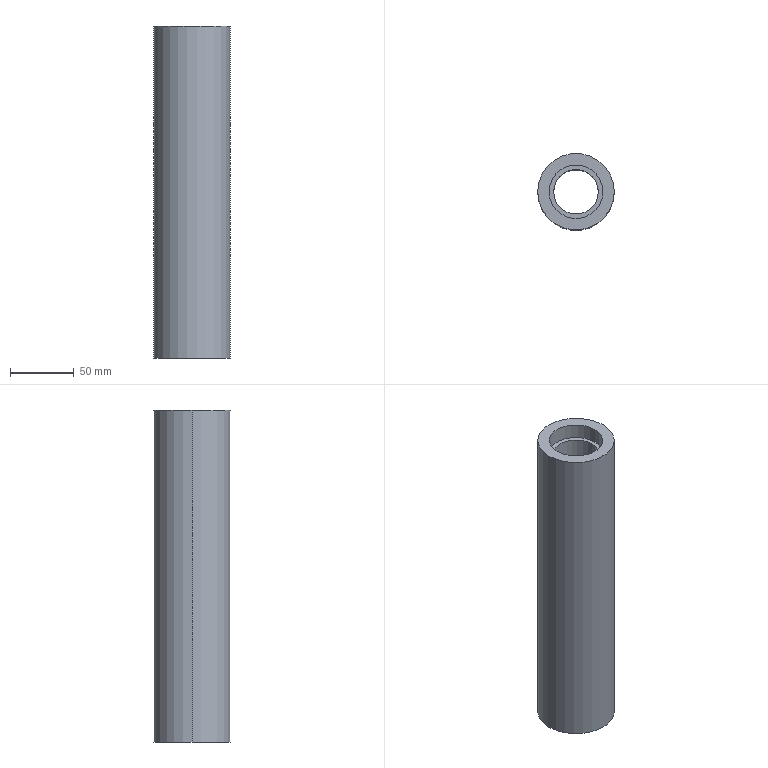Part | SolidWorks | features BaseBody 1 | 1 solid | 12 faces | box 60 x 60 x 260 mm | volume 474823 mm3 | cylinder 8 | plane 4 | commonest cylinder face diameters 42 x4 35 x2 60 x2
STEP:
#1=CARTESIAN_POINT('',(30.,0.,-130.));
#2=VERTEX_POINT('',#1);
#3=CARTESIAN_POINT('',(-30.,0.,-130.));
#4=VERTEX_POINT('',#3);
#5=CARTESIAN_POINT('',(0.,0.,-130.));
#6=DIRECTION('',(0.,0.,1.));
#7=DIRECTION('',(1.,0.,0.));
#8=AXIS2_PLACEMENT_3D('',#5,#6,#7);
#9=CIRCLE('',#8,30.);
#10=EDGE_CURVE('',#2,#4,#9,.T.);
#11=ORIENTED_EDGE('',*,*,#10,.T.);
#12=CARTESIAN_POINT('',(-30.,0.,130.));
#13=VERTEX_POINT('',#12);
#14=CARTESIAN_POINT('',(-30.,0.,-130.));
#15=DIRECTION('',(0.,0.,1.));
#16=VECTOR('',#15,1000.);
#17=LINE('',#14,#16);
#18=EDGE_CURVE('',#4,#13,#17,.T.);
#19=ORIENTED_EDGE('',*,*,#18,.T.);
#20=CARTESIAN_POINT('',(30.,0.,130.));
#21=VERTEX_POINT('',#20);
#22=CARTESIAN_POINT('',(0.,0.,130.));
#23=DIRECTION('',(0.,0.,-1.));
#24=DIRECTION('',(1.,0.,0.));
#25=AXIS2_PLACEMENT_3D('',#22,#23,#24);
#26=CIRCLE('',#25,30.);
#27=EDGE_CURVE('',#13,#21,#26,.T.);
#28=ORIENTED_EDGE('',*,*,#27,.T.);
#29=CARTESIAN_POINT('',(30.,0.,-130.));
#30=DIRECTION('',(0.,0.,1.));
#31=VECTOR('',#30,1000.);
#32=LINE('',#29,#31);
#33=EDGE_CURVE('',#2,#21,#32,.T.);
#34=ORIENTED_EDGE('',*,*,#33,.F.);
#35=EDGE_LOOP('',(#11,#19,#28,#34));
#36=FACE_OUTER_BOUND('',#35,.T.);
#37=CARTESIAN_POINT('',(0.,0.,-130.));
#38=DIRECTION('',(0.,0.,1.));
#39=DIRECTION('',(1.,0.,0.));
#40=AXIS2_PLACEMENT_3D('',#37,#38,#39);
#41=CYLINDRICAL_SURFACE('',#40,30.);
#42=ADVANCED_FACE('',(#36),#41,.T.);
#43=CARTESIAN_POINT('',(21.,0.,-130.));
#44=VERTEX_POINT('',#43);
#45=CARTESIAN_POINT('',(-21.,0.,-130.));
#46=VERTEX_POINT('',#45);
#47=CARTESIAN_POINT('',(0.,0.,-130.));
#48=DIRECTION('',(0.,0.,-1.));
#49=DIRECTION('',(1.,0.,0.));
#50=AXIS2_PLACEMENT_3D('',#47,#48,#49);
#51=CIRCLE('',#50,21.);
#52=EDGE_CURVE('',#44,#46,#51,.T.);
#53=ORIENTED_EDGE('',*,*,#52,.T.);
#54=CARTESIAN_POINT('',(-21.,0.,-118.));
#55=VERTEX_POINT('',#54);
#56=CARTESIAN_POINT('',(-21.,0.,-130.));
#57=DIRECTION('',(0.,0.,1.));
#58=VECTOR('',#57,1000.);
#59=LINE('',#56,#58);
#60=EDGE_CURVE('',#46,#55,#59,.T.);
#61=ORIENTED_EDGE('',*,*,#60,.T.);
#62=CARTESIAN_POINT('',(21.,0.,-118.));
#63=VERTEX_POINT('',#62);
#64=CARTESIAN_POINT('',(0.,0.,-118.));
#65=DIRECTION('',(0.,0.,-1.));
#66=DIRECTION('',(1.,0.,0.));
#67=AXIS2_PLACEMENT_3D('',#64,#65,#66);
#68=CIRCLE('',#67,21.);
#69=EDGE_CURVE('',#63,#55,#68,.T.);
#70=ORIENTED_EDGE('',*,*,#69,.F.);
#71=CARTESIAN_POINT('',(21.,0.,-130.));
#72=DIRECTION('',(0.,0.,1.));
#73=VECTOR('',#72,1000.);
#74=LINE('',#71,#73);
#75=EDGE_CURVE('',#44,#63,#74,.T.);
#76=ORIENTED_EDGE('',*,*,#75,.F.);
#77=EDGE_LOOP('',(#53,#61,#70,#76));
#78=FACE_OUTER_BOUND('',#77,.T.);
#79=CARTESIAN_POINT('',(0.,0.,-130.));
#80=DIRECTION('',(0.,0.,1.));
#81=DIRECTION('',(1.,0.,0.));
#82=AXIS2_PLACEMENT_3D('',#79,#80,#81);
#83=CYLINDRICAL_SURFACE('',#82,21.);
#84=ADVANCED_FACE('',(#78),#83,.F.);
#85=CARTESIAN_POINT('',(-21.,0.,118.));
#86=VERTEX_POINT('',#85);
#87=CARTESIAN_POINT('',(21.,0.,118.));
#88=VERTEX_POINT('',#87);
#89=CARTESIAN_POINT('',(0.,0.,118.));
#90=DIRECTION('',(0.,0.,1.));
#91=DIRECTION('',(1.,0.,0.));
#92=AXIS2_PLACEMENT_3D('',#89,#90,#91);
#93=CIRCLE('',#92,21.);
#94=EDGE_CURVE('',#86,#88,#93,.T.);
#95=ORIENTED_EDGE('',*,*,#94,.F.);
#96=CARTESIAN_POINT('',(-21.,0.,130.));
#97=VERTEX_POINT('',#96);
#98=CARTESIAN_POINT('',(-21.,0.,130.));
#99=DIRECTION('',(0.,0.,1.));
#100=VECTOR('',#99,1000.);
#101=LINE('',#98,#100);
#102=EDGE_CURVE('',#86,#97,#101,.T.);
#103=ORIENTED_EDGE('',*,*,#102,.T.);
#104=CARTESIAN_POINT('',(21.,0.,130.));
#105=VERTEX_POINT('',#104);
#106=CARTESIAN_POINT('',(0.,0.,130.));
#107=DIRECTION('',(0.,0.,-1.));
#108=DIRECTION('',(1.,0.,0.));
#109=AXIS2_PLACEMENT_3D('',#106,#107,#108);
#110=CIRCLE('',#109,21.);
#111=EDGE_CURVE('',#105,#97,#110,.T.);
#112=ORIENTED_EDGE('',*,*,#111,.F.);
#113=CARTESIAN_POINT('',(21.,0.,130.));
#114=DIRECTION('',(0.,0.,1.));
#115=VECTOR('',#114,1000.);
#116=LINE('',#113,#115);
#117=EDGE_CURVE('',#88,#105,#116,.T.);
#118=ORIENTED_EDGE('',*,*,#117,.F.);
#119=EDGE_LOOP('',(#95,#103,#112,#118));
#120=FACE_OUTER_BOUND('',#119,.T.);
#121=CARTESIAN_POINT('',(0.,0.,130.));
#122=DIRECTION('',(0.,0.,1.));
#123=DIRECTION('',(1.,0.,0.));
#124=AXIS2_PLACEMENT_3D('',#121,#122,#123);
#125=CYLINDRICAL_SURFACE('',#124,21.);
#126=ADVANCED_FACE('',(#120),#125,.F.);
#127=CARTESIAN_POINT('',(17.5,0.,-118.));
#128=VERTEX_POINT('',#127);
#129=CARTESIAN_POINT('',(-17.5,0.,-118.));
#130=VERTEX_POINT('',#129);
#131=CARTESIAN_POINT('',(0.,0.,-118.));
#132=DIRECTION('',(0.,0.,-1.));
#133=DIRECTION('',(1.,0.,0.));
#134=AXIS2_PLACEMENT_3D('',#131,#132,#133);
#135=CIRCLE('',#134,17.5);
#136=EDGE_CURVE('',#128,#130,#135,.T.);
#137=ORIENTED_EDGE('',*,*,#136,.T.);
#138=CARTESIAN_POINT('',(-17.5,0.,118.));
#139=VERTEX_POINT('',#138);
#140=CARTESIAN_POINT('',(-17.5,0.,-130.));
#141=DIRECTION('',(0.,0.,1.));
#142=VECTOR('',#141,1000.);
#143=LINE('',#140,#142);
#144=EDGE_CURVE('',#130,#139,#143,.T.);
#145=ORIENTED_EDGE('',*,*,#144,.T.);
#146=CARTESIAN_POINT('',(17.5,0.,118.));
#147=VERTEX_POINT('',#146);
#148=CARTESIAN_POINT('',(0.,0.,118.));
#149=DIRECTION('',(0.,0.,-1.));
#150=DIRECTION('',(1.,0.,0.));
#151=AXIS2_PLACEMENT_3D('',#148,#149,#150);
#152=CIRCLE('',#151,17.5);
#153=EDGE_CURVE('',#147,#139,#152,.T.);
#154=ORIENTED_EDGE('',*,*,#153,.F.);
#155=CARTESIAN_POINT('',(17.5,0.,-130.));
#156=DIRECTION('',(0.,0.,1.));
#157=VECTOR('',#156,1000.);
#158=LINE('',#155,#157);
#159=EDGE_CURVE('',#128,#147,#158,.T.);
#160=ORIENTED_EDGE('',*,*,#159,.F.);
#161=EDGE_LOOP('',(#137,#145,#154,#160));
#162=FACE_OUTER_BOUND('',#161,.T.);
#163=CARTESIAN_POINT('',(0.,0.,-130.));
#164=DIRECTION('',(0.,0.,1.));
#165=DIRECTION('',(1.,0.,0.));
#166=AXIS2_PLACEMENT_3D('',#163,#164,#165);
#167=CYLINDRICAL_SURFACE('',#166,17.5);
#168=ADVANCED_FACE('',(#162),#167,.F.);
#169=ORIENTED_EDGE('',*,*,#18,.F.);
#170=CARTESIAN_POINT('',(0.,0.,-130.));
#171=DIRECTION('',(0.,0.,1.));
#172=DIRECTION('',(1.,0.,0.));
#173=AXIS2_PLACEMENT_3D('',#170,#171,#172);
#174=CIRCLE('',#173,30.);
#175=EDGE_CURVE('',#4,#2,#174,.T.);
#176=ORIENTED_EDGE('',*,*,#175,.T.);
#177=ORIENTED_EDGE('',*,*,#33,.T.);
#178=CARTESIAN_POINT('',(0.,0.,130.));
#179=DIRECTION('',(0.,0.,-1.));
#180=DIRECTION('',(1.,0.,0.));
#181=AXIS2_PLACEMENT_3D('',#178,#179,#180);
#182=CIRCLE('',#181,30.);
#183=EDGE_CURVE('',#21,#13,#182,.T.);
#184=ORIENTED_EDGE('',*,*,#183,.T.);
#185=EDGE_LOOP('',(#169,#176,#177,#184));
#186=FACE_OUTER_BOUND('',#185,.T.);
#187=CARTESIAN_POINT('',(0.,0.,-130.));
#188=DIRECTION('',(0.,0.,1.));
#189=DIRECTION('',(1.,0.,0.));
#190=AXIS2_PLACEMENT_3D('',#187,#188,#189);
#191=CYLINDRICAL_SURFACE('',#190,30.);
#192=ADVANCED_FACE('',(#186),#191,.T.);
#193=ORIENTED_EDGE('',*,*,#52,.F.);
#194=CARTESIAN_POINT('',(0.,0.,-130.));
#195=DIRECTION('',(0.,0.,-1.));
#196=DIRECTION('',(1.,0.,0.));
#197=AXIS2_PLACEMENT_3D('',#194,#195,#196);
#198=CIRCLE('',#197,21.);
#199=EDGE_CURVE('',#46,#44,#198,.T.);
#200=ORIENTED_EDGE('',*,*,#199,.F.);
#201=EDGE_LOOP('',(#193,#200));
#202=FACE_BOUND('',#201,.T.);
#203=ORIENTED_EDGE('',*,*,#10,.F.);
#204=ORIENTED_EDGE('',*,*,#175,.F.);
#205=EDGE_LOOP('',(#203,#204));
#206=FACE_OUTER_BOUND('',#205,.T.);
#207=CARTESIAN_POINT('',(0.,0.,-130.));
#208=DIRECTION('',(0.,0.,1.));
#209=DIRECTION('',(1.,0.,0.));
#210=AXIS2_PLACEMENT_3D('',#207,#208,#209);
#211=PLANE('',#210);
#212=ADVANCED_FACE('',(#202,#206),#211,.F.);
#213=ORIENTED_EDGE('',*,*,#111,.T.);
#214=CARTESIAN_POINT('',(0.,0.,130.));
#215=DIRECTION('',(0.,0.,-1.));
#216=DIRECTION('',(1.,0.,0.));
#217=AXIS2_PLACEMENT_3D('',#214,#215,#216);
#218=CIRCLE('',#217,21.);
#219=EDGE_CURVE('',#97,#105,#218,.T.);
#220=ORIENTED_EDGE('',*,*,#219,.T.);
#221=EDGE_LOOP('',(#213,#220));
#222=FACE_BOUND('',#221,.T.);
#223=ORIENTED_EDGE('',*,*,#183,.F.);
#224=ORIENTED_EDGE('',*,*,#27,.F.);
#225=EDGE_LOOP('',(#223,#224));
#226=FACE_OUTER_BOUND('',#225,.T.);
#227=CARTESIAN_POINT('',(0.,0.,130.));
#228=DIRECTION('',(0.,0.,1.));
#229=DIRECTION('',(1.,0.,0.));
#230=AXIS2_PLACEMENT_3D('',#227,#228,#229);
#231=PLANE('',#230);
#232=ADVANCED_FACE('',(#222,#226),#231,.T.);
#233=ORIENTED_EDGE('',*,*,#60,.F.);
#234=ORIENTED_EDGE('',*,*,#199,.T.);
#235=ORIENTED_EDGE('',*,*,#75,.T.);
#236=CARTESIAN_POINT('',(0.,0.,-118.));
#237=DIRECTION('',(0.,0.,-1.));
#238=DIRECTION('',(1.,0.,0.));
#239=AXIS2_PLACEMENT_3D('',#236,#237,#238);
#240=CIRCLE('',#239,21.);
#241=EDGE_CURVE('',#55,#63,#240,.T.);
#242=ORIENTED_EDGE('',*,*,#241,.F.);
#243=EDGE_LOOP('',(#233,#234,#235,#242));
#244=FACE_OUTER_BOUND('',#243,.T.);
#245=CARTESIAN_POINT('',(0.,0.,-130.));
#246=DIRECTION('',(0.,0.,1.));
#247=DIRECTION('',(1.,0.,0.));
#248=AXIS2_PLACEMENT_3D('',#245,#246,#247);
#249=CYLINDRICAL_SURFACE('',#248,21.);
#250=ADVANCED_FACE('',(#244),#249,.F.);
#251=ORIENTED_EDGE('',*,*,#102,.F.);
#252=CARTESIAN_POINT('',(0.,0.,118.));
#253=DIRECTION('',(0.,0.,1.));
#254=DIRECTION('',(1.,0.,0.));
#255=AXIS2_PLACEMENT_3D('',#252,#253,#254);
#256=CIRCLE('',#255,21.);
#257=EDGE_CURVE('',#88,#86,#256,.T.);
#258=ORIENTED_EDGE('',*,*,#257,.F.);
#259=ORIENTED_EDGE('',*,*,#117,.T.);
#260=ORIENTED_EDGE('',*,*,#219,.F.);
#261=EDGE_LOOP('',(#251,#258,#259,#260));
#262=FACE_OUTER_BOUND('',#261,.T.);
#263=CARTESIAN_POINT('',(0.,0.,130.));
#264=DIRECTION('',(0.,0.,1.));
#265=DIRECTION('',(1.,0.,0.));
#266=AXIS2_PLACEMENT_3D('',#263,#264,#265);
#267=CYLINDRICAL_SURFACE('',#266,21.);
#268=ADVANCED_FACE('',(#262),#267,.F.);
#269=ORIENTED_EDGE('',*,*,#136,.F.);
#270=CARTESIAN_POINT('',(0.,0.,-118.));
#271=DIRECTION('',(0.,0.,-1.));
#272=DIRECTION('',(1.,0.,0.));
#273=AXIS2_PLACEMENT_3D('',#270,#271,#272);
#274=CIRCLE('',#273,17.5);
#275=EDGE_CURVE('',#130,#128,#274,.T.);
#276=ORIENTED_EDGE('',*,*,#275,.F.);
#277=EDGE_LOOP('',(#269,#276));
#278=FACE_BOUND('',#277,.T.);
#279=ORIENTED_EDGE('',*,*,#69,.T.);
#280=ORIENTED_EDGE('',*,*,#241,.T.);
#281=EDGE_LOOP('',(#279,#280));
#282=FACE_OUTER_BOUND('',#281,.T.);
#283=CARTESIAN_POINT('',(0.,0.,-118.));
#284=DIRECTION('',(0.,0.,1.));
#285=DIRECTION('',(1.,0.,0.));
#286=AXIS2_PLACEMENT_3D('',#283,#284,#285);
#287=PLANE('',#286);
#288=ADVANCED_FACE('',(#278,#282),#287,.F.);
#289=ORIENTED_EDGE('',*,*,#153,.T.);
#290=CARTESIAN_POINT('',(0.,0.,118.));
#291=DIRECTION('',(0.,0.,-1.));
#292=DIRECTION('',(1.,0.,0.));
#293=AXIS2_PLACEMENT_3D('',#290,#291,#292);
#294=CIRCLE('',#293,17.5);
#295=EDGE_CURVE('',#139,#147,#294,.T.);
#296=ORIENTED_EDGE('',*,*,#295,.T.);
#297=EDGE_LOOP('',(#289,#296));
#298=FACE_BOUND('',#297,.T.);
#299=ORIENTED_EDGE('',*,*,#257,.T.);
#300=ORIENTED_EDGE('',*,*,#94,.T.);
#301=EDGE_LOOP('',(#299,#300));
#302=FACE_OUTER_BOUND('',#301,.T.);
#303=CARTESIAN_POINT('',(0.,0.,118.));
#304=DIRECTION('',(0.,0.,1.));
#305=DIRECTION('',(1.,0.,0.));
#306=AXIS2_PLACEMENT_3D('',#303,#304,#305);
#307=PLANE('',#306);
#308=ADVANCED_FACE('',(#298,#302),#307,.T.);
#309=ORIENTED_EDGE('',*,*,#144,.F.);
#310=ORIENTED_EDGE('',*,*,#275,.T.);
#311=ORIENTED_EDGE('',*,*,#159,.T.);
#312=ORIENTED_EDGE('',*,*,#295,.F.);
#313=EDGE_LOOP('',(#309,#310,#311,#312));
#314=FACE_OUTER_BOUND('',#313,.T.);
#315=CARTESIAN_POINT('',(0.,0.,-130.));
#316=DIRECTION('',(0.,0.,1.));
#317=DIRECTION('',(1.,0.,0.));
#318=AXIS2_PLACEMENT_3D('',#315,#316,#317);
#319=CYLINDRICAL_SURFACE('',#318,17.5);
#320=ADVANCED_FACE('',(#314),#319,.F.);
#321=CLOSED_SHELL('',(#42,#84,#126,#168,#192,#212,#232,#250,#268,#288,#308,#320));
#322=MANIFOLD_SOLID_BREP('',#321);
#323=CARTESIAN_POINT('',(0.,0.,0.));
#324=DIRECTION('',(0.,0.,1.));
#325=DIRECTION('',(1.,0.,0.));
#326=AXIS2_PLACEMENT_3D('',#323,#324,#325);
#327=(LENGTH_UNIT()NAMED_UNIT(*)SI_UNIT(.MILLI.,.METRE.));
#328=UNCERTAINTY_MEASURE_WITH_UNIT(LENGTH_MEASURE(0.00001),#327,'','');
#329=(NAMED_UNIT(*)PLANE_ANGLE_UNIT()SI_UNIT($,.RADIAN.));
#330=(NAMED_UNIT(*)SI_UNIT($,.STERADIAN.)SOLID_ANGLE_UNIT());
#331=(GEOMETRIC_REPRESENTATION_CONTEXT(3)GLOBAL_UNCERTAINTY_ASSIGNED_CONTEXT((#328))GLOBAL_UNIT_ASSIGNED_CONTEXT((#327,#329,#330))REPRESENTATION_CONTEXT('',''));
#332=ADVANCED_BREP_SHAPE_REPRESENTATION('',(#322,#326),#331);